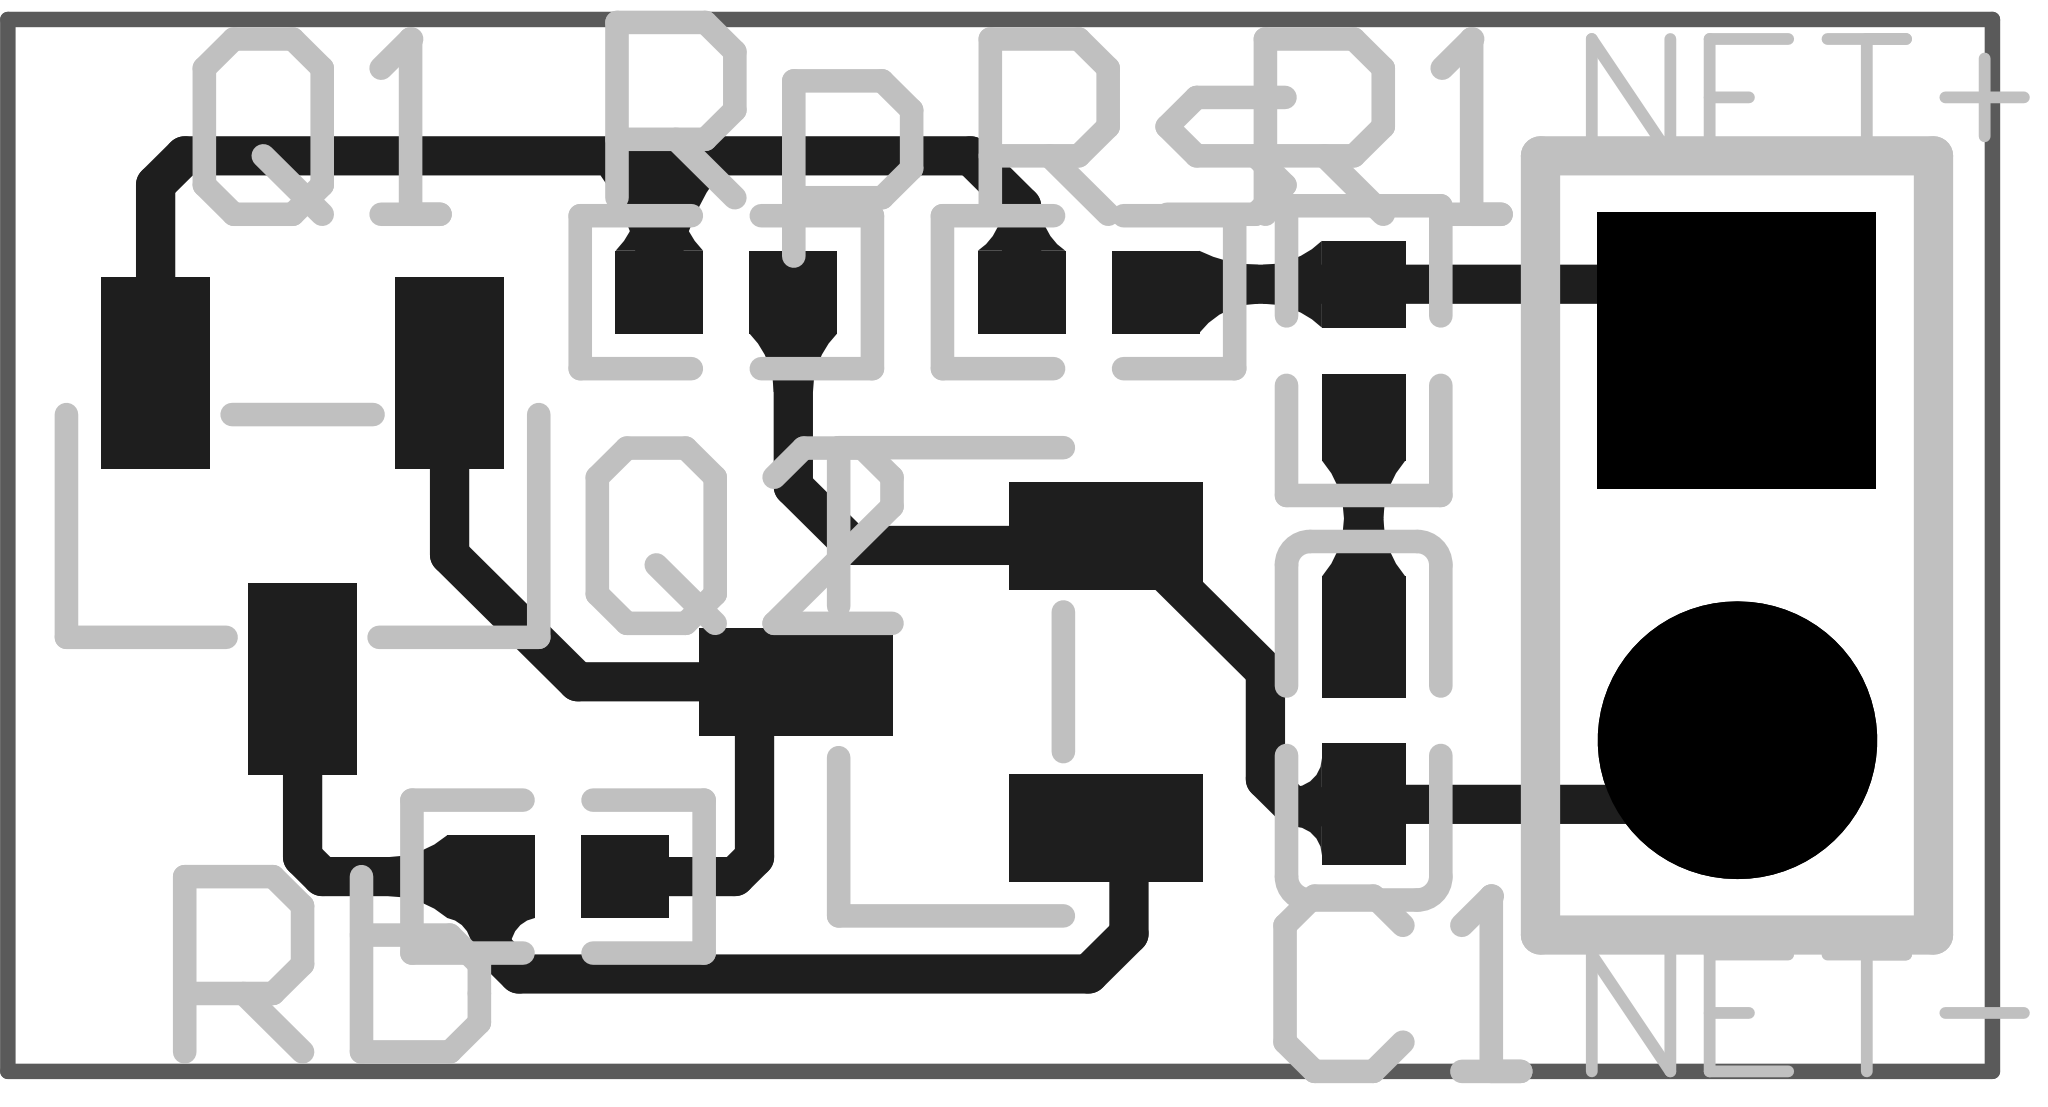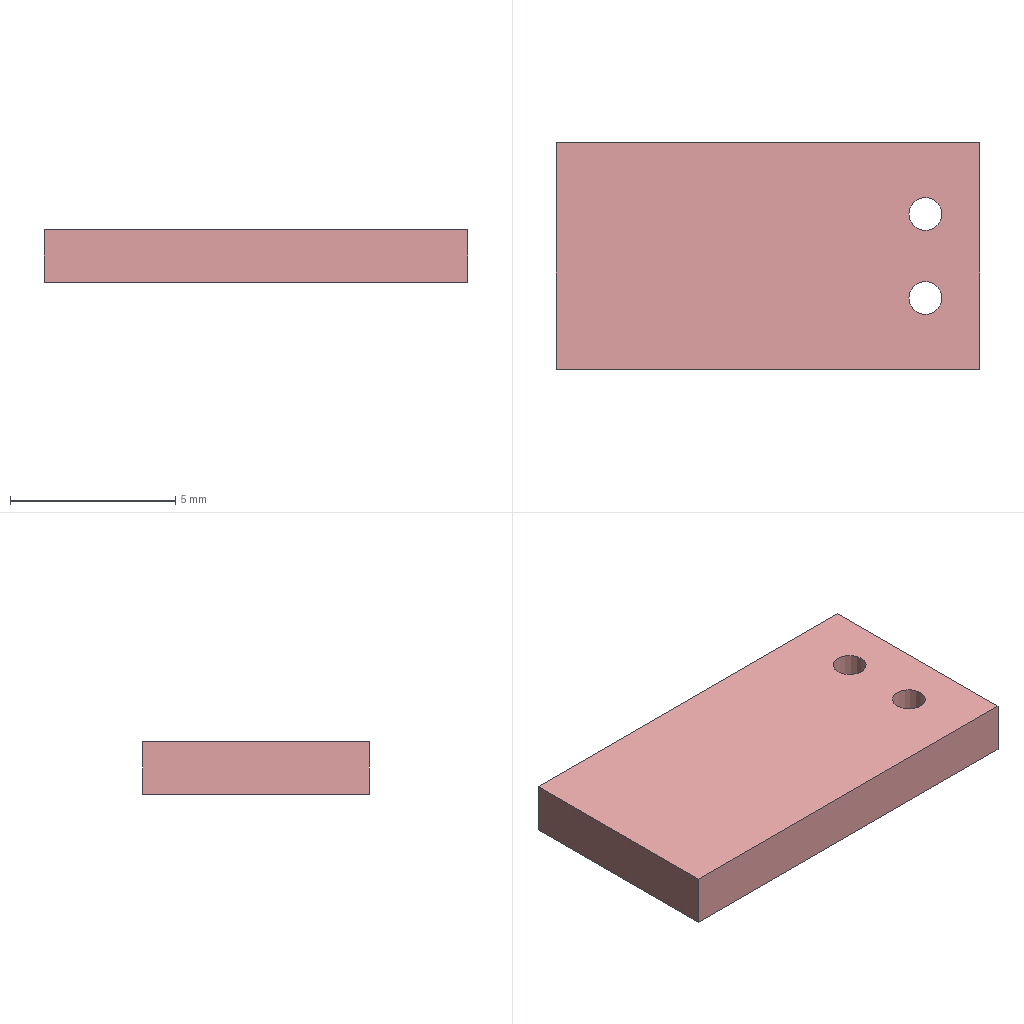Circuit board layout | Altium Designer | box 12.8 x 6.9 x 1.6 mm
Layer stack:
# Altium Designer layer stack of  (unit mm; dielectric type: 0 none, 1 core, 2 prepreg, 3 surface material)
index,name,kind,layer,copper_thickness_mm,dielectric_type,dielectric_thickness_mm,dielectric_material,dielectric_constant
0,Top Paste Mask Layer,other,,,,,,
1,Top Silkscreen Layer,other,,,,,,
2,Top Solder Mask Layer,dielectric,,,3,0.01,,3.3
3,Top Layer,copper,Top Layer,0.035,,,,
4,Dielectric1,dielectric,,,3,1.51,FR4,4.5
5,Bottom Layer,copper,Bottom Layer,0.035,,,,
6,Bottom Solder Mask Layer,dielectric,,,3,0.01,,3.3
7,Bottom Silkscreen Layer,other,,,,,,
8,Bottom Paste Mask Layer,other,,,,,,
# drill layer pairs: low layer,high layer
drill_pair,Top Layer,Bottom Layer
Part placement:
Designator,Comment,Layer,Footprint,Center-X(mm),Center-Y(mm),Rotation
C1,10uF,TopLayer,C0402,84.963,78.486,90
H3,,TopLayer,HDR-TH_2P-P2.54-V-M-1,87.376,79.629,270
R1,0,TopLayer,R0402,84.963,80.899,90
Rb,1K,TopLayer,R0402,79.756,77.47,0
Rp,200K,TopLayer,R0402,80.844,81.28,180
Rs,200,TopLayer,R0402,83.185,81.28,0
Q1,MMBT3906,TopLayer,SOT-23-3_L2.9-W1.3-P1.90-LS2.4-BR,78.105,79.756,90
Q2,MMBT3904,TopLayer,SOT-23-3_L2.9-W1.3-P1.90-LS2.4-BR,82.296,78.74,0
Pad and via stacks:
# Altium Designer via and pad stacks of  (unit mm). Each distinct definition once, with the count of objects using it.
# via: kind,start_layer,end_layer,hole_mm,diameter_mm,mode(0 simple;1 top-mid-bottom;2 full stack),diameter_per_layer,count,example_net
# pad: kind,layer,hole_mm,hole_type(0 round;1 square;2 slot),plating,top_size,top_shape(1 round;2 rect;3 octagon;9 rounded rect),mid_size,bottom_size,mode,footprint,size_per_layer,count,example
pad,Top Layer,0,0,plated,0.7901x0.54,2,0.7901x0.54,0.7901x0.54,0,C0402,,2,C1.2
pad,Top Layer,0,0,plated,0.5657x0.54,2,0.5657x0.54,0.5657x0.54,0,R0402,,8,R1.2
pad,Top Layer,0,0,plated,1.25x0.7,2,1.25x0.7,1.25x0.7,0,SOT-23-3_L2.9-W1.3-P1.90-LS2.4-BR,,6,Q1.1
pad,Multi-Layer,1,0,plated,1.8x1.8,1,1.8x1.8,1.8x1.8,0,HDR-TH_2P-P2.54-V-M-1,,1,H3.2
pad,Multi-Layer,1,0,plated,1.8x1.8,2,1.8x1.8,1.8x1.8,0,HDR-TH_2P-P2.54-V-M-1,,1,H3.1